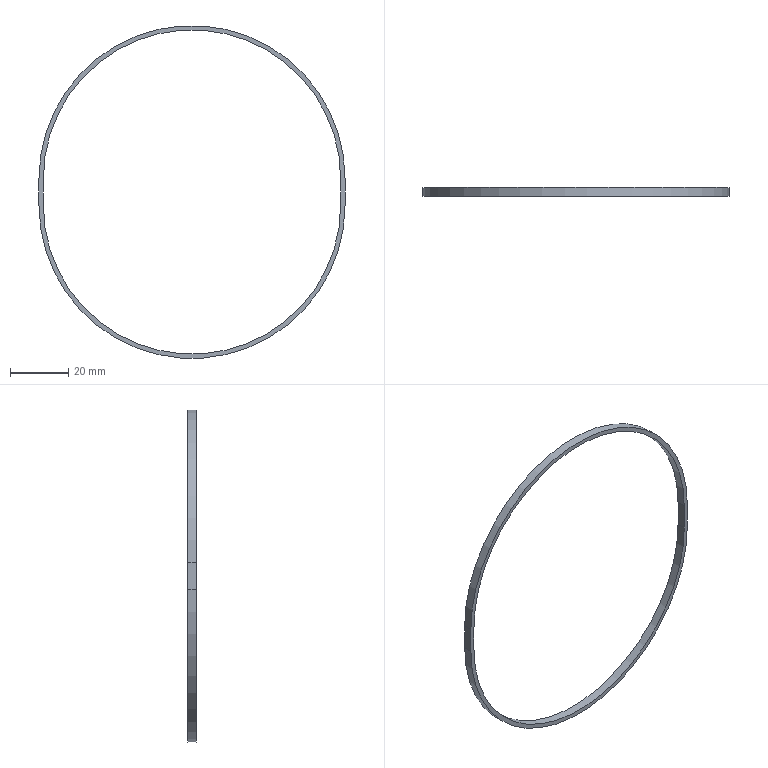Part | STEP file | 1-56.26 | 1 solid | 10 faces | box 105 x 3 x 114.181 mm | volume 1546 mm3 | plane 6 | cylinder 4 | commonest cylinder face diameters 102 x2 105 x2
STEP:
#1=CARTESIAN_POINT('',(0.,0.,0.));
#2=DIRECTION('',(0.,0.,1.));
#3=DIRECTION('',(1.,0.,0.));
#4=AXIS2_PLACEMENT_3D('',#1,#2,#3);
#5=CARTESIAN_POINT('',(-52.5,0.,-9.181));
#6=VERTEX_POINT('',#5);
#7=CARTESIAN_POINT('',(52.5,0.,-9.181));
#8=VERTEX_POINT('',#7);
#9=CARTESIAN_POINT('',(0.,0.,-9.181));
#10=DIRECTION('',(0.,-1.,0.));
#11=DIRECTION('',(-1.,0.,0.));
#12=AXIS2_PLACEMENT_3D('',#9,#10,#11);
#13=CIRCLE('',#12,52.5);
#14=CARTESIAN_POINT('',(4.591,0.,-4.591));
#15=DIRECTION('',(0.,-1.,0.));
#16=DIRECTION('',(1.,0.,0.));
#17=AXIS2_PLACEMENT_3D('',#14,#15,#16);
#18=PLANE('',#17);
#19=CARTESIAN_POINT('',(-4.591,-4.591));
#20=DIRECTION('',(-1.,0.));
#21=AXIS2_PLACEMENT_2D('',#19,#20);
#22=CIRCLE('',#21,52.5);
#23=(GEOMETRIC_REPRESENTATION_CONTEXT(2)PARAMETRIC_REPRESENTATION_CONTEXT()REPRESENTATION_CONTEXT('',''));
#24=DEFINITIONAL_REPRESENTATION('',(#22),#23);
#25=PCURVE('',#18,#24);
#26=CARTESIAN_POINT('',(0.,0.,-9.181));
#27=DIRECTION('',(0.,1.,0.));
#28=DIRECTION('',(-1.,0.,0.));
#29=AXIS2_PLACEMENT_3D('',#26,#27,#28);
#30=CYLINDRICAL_SURFACE('',#29,52.5);
#31=CARTESIAN_POINT('',(6.283,0.));
#32=DIRECTION('',(-1.,0.));
#33=VECTOR('',#32,1.);
#34=LINE('',#31,#33);
#35=(GEOMETRIC_REPRESENTATION_CONTEXT(2)PARAMETRIC_REPRESENTATION_CONTEXT()REPRESENTATION_CONTEXT('',''));
#36=DEFINITIONAL_REPRESENTATION('',(#34),#35);
#37=PCURVE('',#30,#36);
#38=SURFACE_CURVE('',#13,(#25,#37),.PCURVE_S1.);
#39=EDGE_CURVE('',#6,#8,#38,.T.);
#40=ORIENTED_EDGE('',*,*,#39,.T.);
#41=CARTESIAN_POINT('',(52.5,0.,0.));
#42=VERTEX_POINT('',#41);
#43=CARTESIAN_POINT('',(52.5,0.,-9.181));
#44=DIRECTION('',(0.,0.,1.));
#45=VECTOR('',#44,1.);
#46=LINE('',#43,#45);
#47=CARTESIAN_POINT('',(47.909,-4.591));
#48=DIRECTION('',(0.,1.));
#49=VECTOR('',#48,1.);
#50=LINE('',#47,#49);
#51=(GEOMETRIC_REPRESENTATION_CONTEXT(2)PARAMETRIC_REPRESENTATION_CONTEXT()REPRESENTATION_CONTEXT('',''));
#52=DEFINITIONAL_REPRESENTATION('',(#50),#51);
#53=PCURVE('',#18,#52);
#54=CARTESIAN_POINT('',(52.5,1.5,-4.591));
#55=DIRECTION('',(-1.,0.,0.));
#56=DIRECTION('',(0.,0.,1.));
#57=AXIS2_PLACEMENT_3D('',#54,#55,#56);
#58=PLANE('',#57);
#59=CARTESIAN_POINT('',(-4.591,-1.5));
#60=DIRECTION('',(1.,0.));
#61=VECTOR('',#60,1.);
#62=LINE('',#59,#61);
#63=(GEOMETRIC_REPRESENTATION_CONTEXT(2)PARAMETRIC_REPRESENTATION_CONTEXT()REPRESENTATION_CONTEXT('',''));
#64=DEFINITIONAL_REPRESENTATION('',(#62),#63);
#65=PCURVE('',#58,#64);
#66=SURFACE_CURVE('',#46,(#53,#65),.PCURVE_S1.);
#67=EDGE_CURVE('',#8,#42,#66,.T.);
#68=ORIENTED_EDGE('',*,*,#67,.T.);
#69=CARTESIAN_POINT('',(-52.5,0.,0.));
#70=VERTEX_POINT('',#69);
#71=CARTESIAN_POINT('',(0.,0.,0.));
#72=DIRECTION('',(0.,-1.,0.));
#73=DIRECTION('',(1.,0.,0.));
#74=AXIS2_PLACEMENT_3D('',#71,#72,#73);
#75=CIRCLE('',#74,52.5);
#76=CARTESIAN_POINT('',(-4.591,4.591));
#77=DIRECTION('',(1.,0.));
#78=AXIS2_PLACEMENT_2D('',#76,#77);
#79=CIRCLE('',#78,52.5);
#80=(GEOMETRIC_REPRESENTATION_CONTEXT(2)PARAMETRIC_REPRESENTATION_CONTEXT()REPRESENTATION_CONTEXT('',''));
#81=DEFINITIONAL_REPRESENTATION('',(#79),#80);
#82=PCURVE('',#18,#81);
#83=CARTESIAN_POINT('',(0.,0.,0.));
#84=DIRECTION('',(0.,1.,0.));
#85=DIRECTION('',(1.,0.,0.));
#86=AXIS2_PLACEMENT_3D('',#83,#84,#85);
#87=CYLINDRICAL_SURFACE('',#86,52.5);
#88=CARTESIAN_POINT('',(6.283,0.));
#89=DIRECTION('',(-1.,0.));
#90=VECTOR('',#89,1.);
#91=LINE('',#88,#90);
#92=(GEOMETRIC_REPRESENTATION_CONTEXT(2)PARAMETRIC_REPRESENTATION_CONTEXT()REPRESENTATION_CONTEXT('',''));
#93=DEFINITIONAL_REPRESENTATION('',(#91),#92);
#94=PCURVE('',#87,#93);
#95=SURFACE_CURVE('',#75,(#82,#94),.PCURVE_S1.);
#96=EDGE_CURVE('',#42,#70,#95,.T.);
#97=ORIENTED_EDGE('',*,*,#96,.T.);
#98=CARTESIAN_POINT('',(-52.5,0.,0.));
#99=DIRECTION('',(0.,0.,-1.));
#100=VECTOR('',#99,1.);
#101=LINE('',#98,#100);
#102=CARTESIAN_POINT('',(-57.091,4.591));
#103=DIRECTION('',(0.,-1.));
#104=VECTOR('',#103,1.);
#105=LINE('',#102,#104);
#106=(GEOMETRIC_REPRESENTATION_CONTEXT(2)PARAMETRIC_REPRESENTATION_CONTEXT()REPRESENTATION_CONTEXT('',''));
#107=DEFINITIONAL_REPRESENTATION('',(#105),#106);
#108=PCURVE('',#18,#107);
#109=CARTESIAN_POINT('',(-52.5,1.5,-4.591));
#110=DIRECTION('',(1.,0.,0.));
#111=DIRECTION('',(0.,0.,-1.));
#112=AXIS2_PLACEMENT_3D('',#109,#110,#111);
#113=PLANE('',#112);
#114=CARTESIAN_POINT('',(-4.591,-1.5));
#115=DIRECTION('',(1.,0.));
#116=VECTOR('',#115,1.);
#117=LINE('',#114,#116);
#118=(GEOMETRIC_REPRESENTATION_CONTEXT(2)PARAMETRIC_REPRESENTATION_CONTEXT()REPRESENTATION_CONTEXT('',''));
#119=DEFINITIONAL_REPRESENTATION('',(#117),#118);
#120=PCURVE('',#113,#119);
#121=SURFACE_CURVE('',#101,(#108,#120),.PCURVE_S1.);
#122=EDGE_CURVE('',#70,#6,#121,.T.);
#123=ORIENTED_EDGE('',*,*,#122,.T.);
#124=EDGE_LOOP('',(#40,#68,#97,#123));
#125=FACE_BOUND('',#124,.T.);
#126=CARTESIAN_POINT('',(51.,0.,0.));
#127=VERTEX_POINT('',#126);
#128=CARTESIAN_POINT('',(51.,0.,-9.181));
#129=VERTEX_POINT('',#128);
#130=CARTESIAN_POINT('',(51.,0.,0.));
#131=DIRECTION('',(0.,0.,-1.));
#132=VECTOR('',#131,1.);
#133=LINE('',#130,#132);
#134=CARTESIAN_POINT('',(46.409,4.591));
#135=DIRECTION('',(0.,-1.));
#136=VECTOR('',#135,1.);
#137=LINE('',#134,#136);
#138=(GEOMETRIC_REPRESENTATION_CONTEXT(2)PARAMETRIC_REPRESENTATION_CONTEXT()REPRESENTATION_CONTEXT('',''));
#139=DEFINITIONAL_REPRESENTATION('',(#137),#138);
#140=PCURVE('',#18,#139);
#141=CARTESIAN_POINT('',(51.,1.5,-4.591));
#142=DIRECTION('',(1.,0.,0.));
#143=DIRECTION('',(0.,0.,-1.));
#144=AXIS2_PLACEMENT_3D('',#141,#142,#143);
#145=PLANE('',#144);
#146=CARTESIAN_POINT('',(-4.591,-1.5));
#147=DIRECTION('',(1.,0.));
#148=VECTOR('',#147,1.);
#149=LINE('',#146,#148);
#150=(GEOMETRIC_REPRESENTATION_CONTEXT(2)PARAMETRIC_REPRESENTATION_CONTEXT()REPRESENTATION_CONTEXT('',''));
#151=DEFINITIONAL_REPRESENTATION('',(#149),#150);
#152=PCURVE('',#145,#151);
#153=SURFACE_CURVE('',#133,(#140,#152),.PCURVE_S1.);
#154=EDGE_CURVE('',#127,#129,#153,.T.);
#155=ORIENTED_EDGE('',*,*,#154,.T.);
#156=CARTESIAN_POINT('',(-51.,0.,-9.181));
#157=VERTEX_POINT('',#156);
#158=CARTESIAN_POINT('',(0.,0.,-9.181));
#159=DIRECTION('',(0.,1.,0.));
#160=DIRECTION('',(1.,0.,0.));
#161=AXIS2_PLACEMENT_3D('',#158,#159,#160);
#162=CIRCLE('',#161,51.);
#163=CARTESIAN_POINT('',(46.409,-4.591));
#164=CARTESIAN_POINT('',(46.409,-92.925));
#165=CARTESIAN_POINT('',(-30.091,-48.758));
#166=CARTESIAN_POINT('',(-106.591,-4.591));
#167=CARTESIAN_POINT('',(-30.091,39.577));
#168=CARTESIAN_POINT('',(46.409,83.744));
#169=CARTESIAN_POINT('',(46.409,-4.591));
#170=(BOUNDED_CURVE()B_SPLINE_CURVE(2,(#163,#164,#165,#166,#167,#168,#169),.UNSPECIFIED.,.T.,.F.)B_SPLINE_CURVE_WITH_KNOTS((1,2,2,2,2,1),(-2.094,0.,2.094,4.189,6.283,8.378),.UNSPECIFIED.)CURVE()GEOMETRIC_REPRESENTATION_ITEM()RATIONAL_B_SPLINE_CURVE((1.,0.5,1.,0.5,1.,0.5,1.))REPRESENTATION_ITEM(''));
#171=(GEOMETRIC_REPRESENTATION_CONTEXT(2)PARAMETRIC_REPRESENTATION_CONTEXT()REPRESENTATION_CONTEXT('',''));
#172=DEFINITIONAL_REPRESENTATION('',(#170),#171);
#173=PCURVE('',#18,#172);
#174=CARTESIAN_POINT('',(0.,0.,-9.181));
#175=DIRECTION('',(0.,1.,0.));
#176=DIRECTION('',(1.,0.,0.));
#177=AXIS2_PLACEMENT_3D('',#174,#175,#176);
#178=CYLINDRICAL_SURFACE('',#177,51.);
#179=CARTESIAN_POINT('',(0.,0.));
#180=DIRECTION('',(1.,0.));
#181=VECTOR('',#180,1.);
#182=LINE('',#179,#181);
#183=(GEOMETRIC_REPRESENTATION_CONTEXT(2)PARAMETRIC_REPRESENTATION_CONTEXT()REPRESENTATION_CONTEXT('',''));
#184=DEFINITIONAL_REPRESENTATION('',(#182),#183);
#185=PCURVE('',#178,#184);
#186=SURFACE_CURVE('',#162,(#173,#185),.PCURVE_S1.);
#187=EDGE_CURVE('',#129,#157,#186,.T.);
#188=ORIENTED_EDGE('',*,*,#187,.T.);
#189=CARTESIAN_POINT('',(-51.,0.,0.));
#190=VERTEX_POINT('',#189);
#191=CARTESIAN_POINT('',(-51.,0.,-9.181));
#192=DIRECTION('',(0.,0.,1.));
#193=VECTOR('',#192,1.);
#194=LINE('',#191,#193);
#195=CARTESIAN_POINT('',(-55.591,-4.591));
#196=DIRECTION('',(0.,1.));
#197=VECTOR('',#196,1.);
#198=LINE('',#195,#197);
#199=(GEOMETRIC_REPRESENTATION_CONTEXT(2)PARAMETRIC_REPRESENTATION_CONTEXT()REPRESENTATION_CONTEXT('',''));
#200=DEFINITIONAL_REPRESENTATION('',(#198),#199);
#201=PCURVE('',#18,#200);
#202=CARTESIAN_POINT('',(-51.,1.5,-4.591));
#203=DIRECTION('',(-1.,0.,0.));
#204=DIRECTION('',(0.,0.,1.));
#205=AXIS2_PLACEMENT_3D('',#202,#203,#204);
#206=PLANE('',#205);
#207=CARTESIAN_POINT('',(-4.591,-1.5));
#208=DIRECTION('',(1.,0.));
#209=VECTOR('',#208,1.);
#210=LINE('',#207,#209);
#211=(GEOMETRIC_REPRESENTATION_CONTEXT(2)PARAMETRIC_REPRESENTATION_CONTEXT()REPRESENTATION_CONTEXT('',''));
#212=DEFINITIONAL_REPRESENTATION('',(#210),#211);
#213=PCURVE('',#206,#212);
#214=SURFACE_CURVE('',#194,(#201,#213),.PCURVE_S1.);
#215=EDGE_CURVE('',#157,#190,#214,.T.);
#216=ORIENTED_EDGE('',*,*,#215,.T.);
#217=CARTESIAN_POINT('',(0.,0.,0.));
#218=DIRECTION('',(0.,1.,0.));
#219=DIRECTION('',(-1.,0.,0.));
#220=AXIS2_PLACEMENT_3D('',#217,#218,#219);
#221=CIRCLE('',#220,51.);
#222=CARTESIAN_POINT('',(-55.591,4.591));
#223=CARTESIAN_POINT('',(-55.591,92.925));
#224=CARTESIAN_POINT('',(20.909,48.758));
#225=CARTESIAN_POINT('',(97.409,4.591));
#226=CARTESIAN_POINT('',(20.909,-39.577));
#227=CARTESIAN_POINT('',(-55.591,-83.744));
#228=CARTESIAN_POINT('',(-55.591,4.591));
#229=(BOUNDED_CURVE()B_SPLINE_CURVE(2,(#222,#223,#224,#225,#226,#227,#228),.UNSPECIFIED.,.T.,.F.)B_SPLINE_CURVE_WITH_KNOTS((1,2,2,2,2,1),(-2.094,0.,2.094,4.189,6.283,8.378),.UNSPECIFIED.)CURVE()GEOMETRIC_REPRESENTATION_ITEM()RATIONAL_B_SPLINE_CURVE((1.,0.5,1.,0.5,1.,0.5,1.))REPRESENTATION_ITEM(''));
#230=(GEOMETRIC_REPRESENTATION_CONTEXT(2)PARAMETRIC_REPRESENTATION_CONTEXT()REPRESENTATION_CONTEXT('',''));
#231=DEFINITIONAL_REPRESENTATION('',(#229),#230);
#232=PCURVE('',#18,#231);
#233=CARTESIAN_POINT('',(0.,0.,0.));
#234=DIRECTION('',(0.,1.,0.));
#235=DIRECTION('',(-1.,0.,0.));
#236=AXIS2_PLACEMENT_3D('',#233,#234,#235);
#237=CYLINDRICAL_SURFACE('',#236,51.);
#238=CARTESIAN_POINT('',(0.,0.));
#239=DIRECTION('',(1.,0.));
#240=VECTOR('',#239,1.);
#241=LINE('',#238,#240);
#242=(GEOMETRIC_REPRESENTATION_CONTEXT(2)PARAMETRIC_REPRESENTATION_CONTEXT()REPRESENTATION_CONTEXT('',''));
#243=DEFINITIONAL_REPRESENTATION('',(#241),#242);
#244=PCURVE('',#237,#243);
#245=SURFACE_CURVE('',#221,(#232,#244),.PCURVE_S1.);
#246=EDGE_CURVE('',#190,#127,#245,.T.);
#247=ORIENTED_EDGE('',*,*,#246,.T.);
#248=EDGE_LOOP('',(#155,#188,#216,#247));
#249=FACE_BOUND('',#248,.T.);
#250=ADVANCED_FACE('',(#125,#249),#18,.T.);
#251=CARTESIAN_POINT('',(-52.5,3.,-9.181));
#252=VERTEX_POINT('',#251);
#253=CARTESIAN_POINT('',(52.5,3.,-9.181));
#254=VERTEX_POINT('',#253);
#255=CARTESIAN_POINT('',(0.,3.,-9.181));
#256=DIRECTION('',(0.,-1.,0.));
#257=DIRECTION('',(-1.,0.,0.));
#258=AXIS2_PLACEMENT_3D('',#255,#256,#257);
#259=CIRCLE('',#258,52.5);
#260=CARTESIAN_POINT('',(4.591,3.,-4.591));
#261=DIRECTION('',(0.,-1.,0.));
#262=DIRECTION('',(1.,0.,0.));
#263=AXIS2_PLACEMENT_3D('',#260,#261,#262);
#264=PLANE('',#263);
#265=CARTESIAN_POINT('',(-4.591,-4.591));
#266=DIRECTION('',(-1.,0.));
#267=AXIS2_PLACEMENT_2D('',#265,#266);
#268=CIRCLE('',#267,52.5);
#269=(GEOMETRIC_REPRESENTATION_CONTEXT(2)PARAMETRIC_REPRESENTATION_CONTEXT()REPRESENTATION_CONTEXT('',''));
#270=DEFINITIONAL_REPRESENTATION('',(#268),#269);
#271=PCURVE('',#264,#270);
#272=CARTESIAN_POINT('',(6.283,3.));
#273=DIRECTION('',(-1.,0.));
#274=VECTOR('',#273,1.);
#275=LINE('',#272,#274);
#276=(GEOMETRIC_REPRESENTATION_CONTEXT(2)PARAMETRIC_REPRESENTATION_CONTEXT()REPRESENTATION_CONTEXT('',''));
#277=DEFINITIONAL_REPRESENTATION('',(#275),#276);
#278=PCURVE('',#30,#277);
#279=SURFACE_CURVE('',#259,(#271,#278),.PCURVE_S1.);
#280=EDGE_CURVE('',#252,#254,#279,.T.);
#281=ORIENTED_EDGE('',*,*,#280,.T.);
#282=CARTESIAN_POINT('',(52.5,3.,0.));
#283=VERTEX_POINT('',#282);
#284=CARTESIAN_POINT('',(52.5,3.,-9.181));
#285=DIRECTION('',(0.,0.,1.));
#286=VECTOR('',#285,1.);
#287=LINE('',#284,#286);
#288=CARTESIAN_POINT('',(47.909,-4.591));
#289=DIRECTION('',(0.,1.));
#290=VECTOR('',#289,1.);
#291=LINE('',#288,#290);
#292=(GEOMETRIC_REPRESENTATION_CONTEXT(2)PARAMETRIC_REPRESENTATION_CONTEXT()REPRESENTATION_CONTEXT('',''));
#293=DEFINITIONAL_REPRESENTATION('',(#291),#292);
#294=PCURVE('',#264,#293);
#295=CARTESIAN_POINT('',(-4.591,1.5));
#296=DIRECTION('',(1.,0.));
#297=VECTOR('',#296,1.);
#298=LINE('',#295,#297);
#299=(GEOMETRIC_REPRESENTATION_CONTEXT(2)PARAMETRIC_REPRESENTATION_CONTEXT()REPRESENTATION_CONTEXT('',''));
#300=DEFINITIONAL_REPRESENTATION('',(#298),#299);
#301=PCURVE('',#58,#300);
#302=SURFACE_CURVE('',#287,(#294,#301),.PCURVE_S1.);
#303=EDGE_CURVE('',#254,#283,#302,.T.);
#304=ORIENTED_EDGE('',*,*,#303,.T.);
#305=CARTESIAN_POINT('',(-52.5,3.,0.));
#306=VERTEX_POINT('',#305);
#307=CARTESIAN_POINT('',(0.,3.,0.));
#308=DIRECTION('',(0.,-1.,0.));
#309=DIRECTION('',(1.,0.,0.));
#310=AXIS2_PLACEMENT_3D('',#307,#308,#309);
#311=CIRCLE('',#310,52.5);
#312=CARTESIAN_POINT('',(-4.591,4.591));
#313=DIRECTION('',(1.,0.));
#314=AXIS2_PLACEMENT_2D('',#312,#313);
#315=CIRCLE('',#314,52.5);
#316=(GEOMETRIC_REPRESENTATION_CONTEXT(2)PARAMETRIC_REPRESENTATION_CONTEXT()REPRESENTATION_CONTEXT('',''));
#317=DEFINITIONAL_REPRESENTATION('',(#315),#316);
#318=PCURVE('',#264,#317);
#319=CARTESIAN_POINT('',(6.283,3.));
#320=DIRECTION('',(-1.,0.));
#321=VECTOR('',#320,1.);
#322=LINE('',#319,#321);
#323=(GEOMETRIC_REPRESENTATION_CONTEXT(2)PARAMETRIC_REPRESENTATION_CONTEXT()REPRESENTATION_CONTEXT('',''));
#324=DEFINITIONAL_REPRESENTATION('',(#322),#323);
#325=PCURVE('',#87,#324);
#326=SURFACE_CURVE('',#311,(#318,#325),.PCURVE_S1.);
#327=EDGE_CURVE('',#283,#306,#326,.T.);
#328=ORIENTED_EDGE('',*,*,#327,.T.);
#329=CARTESIAN_POINT('',(-52.5,3.,0.));
#330=DIRECTION('',(0.,0.,-1.));
#331=VECTOR('',#330,1.);
#332=LINE('',#329,#331);
#333=CARTESIAN_POINT('',(-57.091,4.591));
#334=DIRECTION('',(0.,-1.));
#335=VECTOR('',#334,1.);
#336=LINE('',#333,#335);
#337=(GEOMETRIC_REPRESENTATION_CONTEXT(2)PARAMETRIC_REPRESENTATION_CONTEXT()REPRESENTATION_CONTEXT('',''));
#338=DEFINITIONAL_REPRESENTATION('',(#336),#337);
#339=PCURVE('',#264,#338);
#340=CARTESIAN_POINT('',(-4.591,1.5));
#341=DIRECTION('',(1.,0.));
#342=VECTOR('',#341,1.);
#343=LINE('',#340,#342);
#344=(GEOMETRIC_REPRESENTATION_CONTEXT(2)PARAMETRIC_REPRESENTATION_CONTEXT()REPRESENTATION_CONTEXT('',''));
#345=DEFINITIONAL_REPRESENTATION('',(#343),#344);
#346=PCURVE('',#113,#345);
#347=SURFACE_CURVE('',#332,(#339,#346),.PCURVE_S1.);
#348=EDGE_CURVE('',#306,#252,#347,.T.);
#349=ORIENTED_EDGE('',*,*,#348,.T.);
#350=EDGE_LOOP('',(#281,#304,#328,#349));
#351=FACE_BOUND('',#350,.F.);
#352=CARTESIAN_POINT('',(51.,3.,0.));
#353=VERTEX_POINT('',#352);
#354=CARTESIAN_POINT('',(51.,3.,-9.181));
#355=VERTEX_POINT('',#354);
#356=CARTESIAN_POINT('',(51.,3.,0.));
#357=DIRECTION('',(0.,0.,-1.));
#358=VECTOR('',#357,1.);
#359=LINE('',#356,#358);
#360=CARTESIAN_POINT('',(46.409,4.591));
#361=DIRECTION('',(0.,-1.));
#362=VECTOR('',#361,1.);
#363=LINE('',#360,#362);
#364=(GEOMETRIC_REPRESENTATION_CONTEXT(2)PARAMETRIC_REPRESENTATION_CONTEXT()REPRESENTATION_CONTEXT('',''));
#365=DEFINITIONAL_REPRESENTATION('',(#363),#364);
#366=PCURVE('',#264,#365);
#367=CARTESIAN_POINT('',(-4.591,1.5));
#368=DIRECTION('',(1.,0.));
#369=VECTOR('',#368,1.);
#370=LINE('',#367,#369);
#371=(GEOMETRIC_REPRESENTATION_CONTEXT(2)PARAMETRIC_REPRESENTATION_CONTEXT()REPRESENTATION_CONTEXT('',''));
#372=DEFINITIONAL_REPRESENTATION('',(#370),#371);
#373=PCURVE('',#145,#372);
#374=SURFACE_CURVE('',#359,(#366,#373),.PCURVE_S1.);
#375=EDGE_CURVE('',#353,#355,#374,.T.);
#376=ORIENTED_EDGE('',*,*,#375,.T.);
#377=CARTESIAN_POINT('',(-51.,3.,-9.181));
#378=VERTEX_POINT('',#377);
#379=CARTESIAN_POINT('',(0.,3.,-9.181));
#380=DIRECTION('',(0.,1.,0.));
#381=DIRECTION('',(1.,0.,0.));
#382=AXIS2_PLACEMENT_3D('',#379,#380,#381);
#383=CIRCLE('',#382,51.);
#384=CARTESIAN_POINT('',(46.409,-4.591));
#385=CARTESIAN_POINT('',(46.409,-92.925));
#386=CARTESIAN_POINT('',(-30.091,-48.758));
#387=CARTESIAN_POINT('',(-106.591,-4.591));
#388=CARTESIAN_POINT('',(-30.091,39.577));
#389=CARTESIAN_POINT('',(46.409,83.744));
#390=CARTESIAN_POINT('',(46.409,-4.591));
#391=(BOUNDED_CURVE()B_SPLINE_CURVE(2,(#384,#385,#386,#387,#388,#389,#390),.UNSPECIFIED.,.T.,.F.)B_SPLINE_CURVE_WITH_KNOTS((1,2,2,2,2,1),(-2.094,0.,2.094,4.189,6.283,8.378),.UNSPECIFIED.)CURVE()GEOMETRIC_REPRESENTATION_ITEM()RATIONAL_B_SPLINE_CURVE((1.,0.5,1.,0.5,1.,0.5,1.))REPRESENTATION_ITEM(''));
#392=(GEOMETRIC_REPRESENTATION_CONTEXT(2)PARAMETRIC_REPRESENTATION_CONTEXT()REPRESENTATION_CONTEXT('',''));
#393=DEFINITIONAL_REPRESENTATION('',(#391),#392);
#394=PCURVE('',#264,#393);
#395=CARTESIAN_POINT('',(0.,3.));
#396=DIRECTION('',(1.,0.));
#397=VECTOR('',#396,1.);
#398=LINE('',#395,#397);
#399=(GEOMETRIC_REPRESENTATION_CONTEXT(2)PARAMETRIC_REPRESENTATION_CONTEXT()REPRESENTATION_CONTEXT('',''));
#400=DEFINITIONAL_REPRESENTATION('',(#398),#399);
#401=PCURVE('',#178,#400);
#402=SURFACE_CURVE('',#383,(#394,#401),.PCURVE_S1.);
#403=EDGE_CURVE('',#355,#378,#402,.T.);
#404=ORIENTED_EDGE('',*,*,#403,.T.);
#405=CARTESIAN_POINT('',(-51.,3.,0.));
#406=VERTEX_POINT('',#405);
#407=CARTESIAN_POINT('',(-51.,3.,-9.181));
#408=DIRECTION('',(0.,0.,1.));
#409=VECTOR('',#408,1.);
#410=LINE('',#407,#409);
#411=CARTESIAN_POINT('',(-55.591,-4.591));
#412=DIRECTION('',(0.,1.));
#413=VECTOR('',#412,1.);
#414=LINE('',#411,#413);
#415=(GEOMETRIC_REPRESENTATION_CONTEXT(2)PARAMETRIC_REPRESENTATION_CONTEXT()REPRESENTATION_CONTEXT('',''));
#416=DEFINITIONAL_REPRESENTATION('',(#414),#415);
#417=PCURVE('',#264,#416);
#418=CARTESIAN_POINT('',(-4.591,1.5));
#419=DIRECTION('',(1.,0.));
#420=VECTOR('',#419,1.);
#421=LINE('',#418,#420);
#422=(GEOMETRIC_REPRESENTATION_CONTEXT(2)PARAMETRIC_REPRESENTATION_CONTEXT()REPRESENTATION_CONTEXT('',''));
#423=DEFINITIONAL_REPRESENTATION('',(#421),#422);
#424=PCURVE('',#206,#423);
#425=SURFACE_CURVE('',#410,(#417,#424),.PCURVE_S1.);
#426=EDGE_CURVE('',#378,#406,#425,.T.);
#427=ORIENTED_EDGE('',*,*,#426,.T.);
#428=CARTESIAN_POINT('',(0.,3.,0.));
#429=DIRECTION('',(0.,1.,0.));
#430=DIRECTION('',(-1.,0.,0.));
#431=AXIS2_PLACEMENT_3D('',#428,#429,#430);
#432=CIRCLE('',#431,51.);
#433=CARTESIAN_POINT('',(-55.591,4.591));
#434=CARTESIAN_POINT('',(-55.591,92.925));
#435=CARTESIAN_POINT('',(20.909,48.758));
#436=CARTESIAN_POINT('',(97.409,4.591));
#437=CARTESIAN_POINT('',(20.909,-39.577));
#438=CARTESIAN_POINT('',(-55.591,-83.744));
#439=CARTESIAN_POINT('',(-55.591,4.591));
#440=(BOUNDED_CURVE()B_SPLINE_CURVE(2,(#433,#434,#435,#436,#437,#438,#439),.UNSPECIFIED.,.T.,.F.)B_SPLINE_CURVE_WITH_KNOTS((1,2,2,2,2,1),(-2.094,0.,2.094,4.189,6.283,8.378),.UNSPECIFIED.)CURVE()GEOMETRIC_REPRESENTATION_ITEM()RATIONAL_B_SPLINE_CURVE((1.,0.5,1.,0.5,1.,0.5,1.))REPRESENTATION_ITEM(''));
#441=(GEOMETRIC_REPRESENTATION_CONTEXT(2)PARAMETRIC_REPRESENTATION_CONTEXT()REPRESENTATION_CONTEXT('',''));
#442=DEFINITIONAL_REPRESENTATION('',(#440),#441);
#443=PCURVE('',#264,#442);
#444=CARTESIAN_POINT('',(0.,3.));
#445=DIRECTION('',(1.,0.));
#446=VECTOR('',#445,1.);
#447=LINE('',#444,#446);
#448=(GEOMETRIC_REPRESENTATION_CONTEXT(2)PARAMETRIC_REPRESENTATION_CONTEXT()REPRESENTATION_CONTEXT('',''));
#449=DEFINITIONAL_REPRESENTATION('',(#447),#448);
#450=PCURVE('',#237,#449);
#451=SURFACE_CURVE('',#432,(#443,#450),.PCURVE_S1.);
#452=EDGE_CURVE('',#406,#353,#451,.T.);
#453=ORIENTED_EDGE('',*,*,#452,.T.);
#454=EDGE_LOOP('',(#376,#404,#427,#453));
#455=FACE_BOUND('',#454,.F.);
#456=ADVANCED_FACE('',(#351,#455),#264,.F.);
#457=CARTESIAN_POINT('',(-52.5,0.,-9.181));
#458=DIRECTION('',(0.,1.,0.));
#459=VECTOR('',#458,1.);
#460=LINE('',#457,#459);
#461=CARTESIAN_POINT('',(6.283,0.));
#462=DIRECTION('',(0.,1.));
#463=VECTOR('',#462,1.);
#464=LINE('',#461,#463);
#465=(GEOMETRIC_REPRESENTATION_CONTEXT(2)PARAMETRIC_REPRESENTATION_CONTEXT()REPRESENTATION_CONTEXT('',''));
#466=DEFINITIONAL_REPRESENTATION('',(#464),#465);
#467=PCURVE('',#30,#466);
#468=CARTESIAN_POINT('',(4.591,-1.5));
#469=DIRECTION('',(0.,1.));
#470=VECTOR('',#469,1.);
#471=LINE('',#468,#470);
#472=(GEOMETRIC_REPRESENTATION_CONTEXT(2)PARAMETRIC_REPRESENTATION_CONTEXT()REPRESENTATION_CONTEXT('',''));
#473=DEFINITIONAL_REPRESENTATION('',(#471),#472);
#474=PCURVE('',#113,#473);
#475=SURFACE_CURVE('',#460,(#467,#474),.PCURVE_S1.);
#476=EDGE_CURVE('',#6,#252,#475,.T.);
#477=ORIENTED_EDGE('',*,*,#476,.T.);
#478=ORIENTED_EDGE('',*,*,#280,.T.);
#479=CARTESIAN_POINT('',(52.5,0.,-9.181));
#480=DIRECTION('',(0.,1.,0.));
#481=VECTOR('',#480,1.);
#482=LINE('',#479,#481);
#483=CARTESIAN_POINT('',(3.142,0.));
#484=DIRECTION('',(0.,1.));
#485=VECTOR('',#484,1.);
#486=LINE('',#483,#485);
#487=(GEOMETRIC_REPRESENTATION_CONTEXT(2)PARAMETRIC_REPRESENTATION_CONTEXT()REPRESENTATION_CONTEXT('',''));
#488=DEFINITIONAL_REPRESENTATION('',(#486),#487);
#489=PCURVE('',#30,#488);
#490=CARTESIAN_POINT('',(-4.591,-1.5));
#491=DIRECTION('',(0.,1.));
#492=VECTOR('',#491,1.);
#493=LINE('',#490,#492);
#494=(GEOMETRIC_REPRESENTATION_CONTEXT(2)PARAMETRIC_REPRESENTATION_CONTEXT()REPRESENTATION_CONTEXT('',''));
#495=DEFINITIONAL_REPRESENTATION('',(#493),#494);
#496=PCURVE('',#58,#495);
#497=SURFACE_CURVE('',#482,(#489,#496),.PCURVE_S1.);
#498=EDGE_CURVE('',#8,#254,#497,.T.);
#499=ORIENTED_EDGE('',*,*,#498,.F.);
#500=ORIENTED_EDGE('',*,*,#39,.F.);
#501=EDGE_LOOP('',(#477,#478,#499,#500));
#502=FACE_BOUND('',#501,.T.);
#503=ADVANCED_FACE('',(#502),#30,.T.);
#504=ORIENTED_EDGE('',*,*,#67,.T.);
#505=CARTESIAN_POINT('',(52.5,0.,0.));
#506=DIRECTION('',(0.,1.,0.));
#507=VECTOR('',#506,1.);
#508=LINE('',#505,#507);
#509=CARTESIAN_POINT('',(4.591,-1.5));
#510=DIRECTION('',(0.,1.));
#511=VECTOR('',#510,1.);
#512=LINE('',#509,#511);
#513=(GEOMETRIC_REPRESENTATION_CONTEXT(2)PARAMETRIC_REPRESENTATION_CONTEXT()REPRESENTATION_CONTEXT('',''));
#514=DEFINITIONAL_REPRESENTATION('',(#512),#513);
#515=PCURVE('',#58,#514);
#516=CARTESIAN_POINT('',(6.283,0.));
#517=DIRECTION('',(0.,1.));
#518=VECTOR('',#517,1.);
#519=LINE('',#516,#518);
#520=(GEOMETRIC_REPRESENTATION_CONTEXT(2)PARAMETRIC_REPRESENTATION_CONTEXT()REPRESENTATION_CONTEXT('',''));
#521=DEFINITIONAL_REPRESENTATION('',(#519),#520);
#522=PCURVE('',#87,#521);
#523=SURFACE_CURVE('',#508,(#515,#522),.PCURVE_S1.);
#524=EDGE_CURVE('',#42,#283,#523,.T.);
#525=ORIENTED_EDGE('',*,*,#524,.T.);
#526=ORIENTED_EDGE('',*,*,#303,.F.);
#527=ORIENTED_EDGE('',*,*,#498,.F.);
#528=EDGE_LOOP('',(#504,#525,#526,#527));
#529=FACE_BOUND('',#528,.F.);
#530=ADVANCED_FACE('',(#529),#58,.F.);
#531=ORIENTED_EDGE('',*,*,#524,.T.);
#532=ORIENTED_EDGE('',*,*,#327,.T.);
#533=CARTESIAN_POINT('',(-52.5,0.,0.));
#534=DIRECTION('',(0.,1.,0.));
#535=VECTOR('',#534,1.);
#536=LINE('',#533,#535);
#537=CARTESIAN_POINT('',(3.142,0.));
#538=DIRECTION('',(0.,1.));
#539=VECTOR('',#538,1.);
#540=LINE('',#537,#539);
#541=(GEOMETRIC_REPRESENTATION_CONTEXT(2)PARAMETRIC_REPRESENTATION_CONTEXT()REPRESENTATION_CONTEXT('',''));
#542=DEFINITIONAL_REPRESENTATION('',(#540),#541);
#543=PCURVE('',#87,#542);
#544=CARTESIAN_POINT('',(-4.591,-1.5));
#545=DIRECTION('',(0.,1.));
#546=VECTOR('',#545,1.);
#547=LINE('',#544,#546);
#548=(GEOMETRIC_REPRESENTATION_CONTEXT(2)PARAMETRIC_REPRESENTATION_CONTEXT()REPRESENTATION_CONTEXT('',''));
#549=DEFINITIONAL_REPRESENTATION('',(#547),#548);
#550=PCURVE('',#113,#549);
#551=SURFACE_CURVE('',#536,(#543,#550),.PCURVE_S1.);
#552=EDGE_CURVE('',#70,#306,#551,.T.);
#553=ORIENTED_EDGE('',*,*,#552,.F.);
#554=ORIENTED_EDGE('',*,*,#96,.F.);
#555=EDGE_LOOP('',(#531,#532,#553,#554));
#556=FACE_BOUND('',#555,.T.);
#557=ADVANCED_FACE('',(#556),#87,.T.);
#558=ORIENTED_EDGE('',*,*,#122,.T.);
#559=ORIENTED_EDGE('',*,*,#476,.T.);
#560=ORIENTED_EDGE('',*,*,#348,.F.);
#561=ORIENTED_EDGE('',*,*,#552,.F.);
#562=EDGE_LOOP('',(#558,#559,#560,#561));
#563=FACE_BOUND('',#562,.F.);
#564=ADVANCED_FACE('',(#563),#113,.F.);
#565=ORIENTED_EDGE('',*,*,#154,.T.);
#566=CARTESIAN_POINT('',(51.,0.,-9.181));
#567=DIRECTION('',(0.,1.,0.));
#568=VECTOR('',#567,1.);
#569=LINE('',#566,#568);
#570=CARTESIAN_POINT('',(4.591,-1.5));
#571=DIRECTION('',(0.,1.));
#572=VECTOR('',#571,1.);
#573=LINE('',#570,#572);
#574=(GEOMETRIC_REPRESENTATION_CONTEXT(2)PARAMETRIC_REPRESENTATION_CONTEXT()REPRESENTATION_CONTEXT('',''));
#575=DEFINITIONAL_REPRESENTATION('',(#573),#574);
#576=PCURVE('',#145,#575);
#577=CARTESIAN_POINT('',(0.,0.));
#578=DIRECTION('',(0.,1.));
#579=VECTOR('',#578,1.);
#580=LINE('',#577,#579);
#581=(GEOMETRIC_REPRESENTATION_CONTEXT(2)PARAMETRIC_REPRESENTATION_CONTEXT()REPRESENTATION_CONTEXT('',''));
#582=DEFINITIONAL_REPRESENTATION('',(#580),#581);
#583=PCURVE('',#178,#582);
#584=SURFACE_CURVE('',#569,(#576,#583),.PCURVE_S1.);
#585=EDGE_CURVE('',#129,#355,#584,.T.);
#586=ORIENTED_EDGE('',*,*,#585,.T.);
#587=ORIENTED_EDGE('',*,*,#375,.F.);
#588=CARTESIAN_POINT('',(51.,0.,0.));
#589=DIRECTION('',(0.,1.,0.));
#590=VECTOR('',#589,1.);
#591=LINE('',#588,#590);
#592=CARTESIAN_POINT('',(-4.591,-1.5));
#593=DIRECTION('',(0.,1.));
#594=VECTOR('',#593,1.);
#595=LINE('',#592,#594);
#596=(GEOMETRIC_REPRESENTATION_CONTEXT(2)PARAMETRIC_REPRESENTATION_CONTEXT()REPRESENTATION_CONTEXT('',''));
#597=DEFINITIONAL_REPRESENTATION('',(#595),#596);
#598=PCURVE('',#145,#597);
#599=CARTESIAN_POINT('',(3.142,0.));
#600=DIRECTION('',(0.,1.));
#601=VECTOR('',#600,1.);
#602=LINE('',#599,#601);
#603=(GEOMETRIC_REPRESENTATION_CONTEXT(2)PARAMETRIC_REPRESENTATION_CONTEXT()REPRESENTATION_CONTEXT('',''));
#604=DEFINITIONAL_REPRESENTATION('',(#602),#603);
#605=PCURVE('',#237,#604);
#606=SURFACE_CURVE('',#591,(#598,#605),.PCURVE_S1.);
#607=EDGE_CURVE('',#127,#353,#606,.T.);
#608=ORIENTED_EDGE('',*,*,#607,.F.);
#609=EDGE_LOOP('',(#565,#586,#587,#608));
#610=FACE_BOUND('',#609,.F.);
#611=ADVANCED_FACE('',(#610),#145,.F.);
#612=ORIENTED_EDGE('',*,*,#187,.T.);
#613=CARTESIAN_POINT('',(-51.,0.,-9.181));
#614=DIRECTION('',(0.,1.,0.));
#615=VECTOR('',#614,1.);
#616=LINE('',#613,#615);
#617=CARTESIAN_POINT('',(3.142,0.));
#618=DIRECTION('',(0.,1.));
#619=VECTOR('',#618,1.);
#620=LINE('',#617,#619);
#621=(GEOMETRIC_REPRESENTATION_CONTEXT(2)PARAMETRIC_REPRESENTATION_CONTEXT()REPRESENTATION_CONTEXT('',''));
#622=DEFINITIONAL_REPRESENTATION('',(#620),#621);
#623=PCURVE('',#178,#622);
#624=CARTESIAN_POINT('',(-4.591,-1.5));
#625=DIRECTION('',(0.,1.));
#626=VECTOR('',#625,1.);
#627=LINE('',#624,#626);
#628=(GEOMETRIC_REPRESENTATION_CONTEXT(2)PARAMETRIC_REPRESENTATION_CONTEXT()REPRESENTATION_CONTEXT('',''));
#629=DEFINITIONAL_REPRESENTATION('',(#627),#628);
#630=PCURVE('',#206,#629);
#631=SURFACE_CURVE('',#616,(#623,#630),.PCURVE_S1.);
#632=EDGE_CURVE('',#157,#378,#631,.T.);
#633=ORIENTED_EDGE('',*,*,#632,.T.);
#634=ORIENTED_EDGE('',*,*,#403,.F.);
#635=ORIENTED_EDGE('',*,*,#585,.F.);
#636=EDGE_LOOP('',(#612,#633,#634,#635));
#637=FACE_BOUND('',#636,.F.);
#638=ADVANCED_FACE('',(#637),#178,.F.);
#639=ORIENTED_EDGE('',*,*,#215,.T.);
#640=CARTESIAN_POINT('',(-51.,0.,0.));
#641=DIRECTION('',(0.,1.,0.));
#642=VECTOR('',#641,1.);
#643=LINE('',#640,#642);
#644=CARTESIAN_POINT('',(4.591,-1.5));
#645=DIRECTION('',(0.,1.));
#646=VECTOR('',#645,1.);
#647=LINE('',#644,#646);
#648=(GEOMETRIC_REPRESENTATION_CONTEXT(2)PARAMETRIC_REPRESENTATION_CONTEXT()REPRESENTATION_CONTEXT('',''));
#649=DEFINITIONAL_REPRESENTATION('',(#647),#648);
#650=PCURVE('',#206,#649);
#651=CARTESIAN_POINT('',(0.,0.));
#652=DIRECTION('',(0.,1.));
#653=VECTOR('',#652,1.);
#654=LINE('',#651,#653);
#655=(GEOMETRIC_REPRESENTATION_CONTEXT(2)PARAMETRIC_REPRESENTATION_CONTEXT()REPRESENTATION_CONTEXT('',''));
#656=DEFINITIONAL_REPRESENTATION('',(#654),#655);
#657=PCURVE('',#237,#656);
#658=SURFACE_CURVE('',#643,(#650,#657),.PCURVE_S1.);
#659=EDGE_CURVE('',#190,#406,#658,.T.);
#660=ORIENTED_EDGE('',*,*,#659,.T.);
#661=ORIENTED_EDGE('',*,*,#426,.F.);
#662=ORIENTED_EDGE('',*,*,#632,.F.);
#663=EDGE_LOOP('',(#639,#660,#661,#662));
#664=FACE_BOUND('',#663,.F.);
#665=ADVANCED_FACE('',(#664),#206,.F.);
#666=ORIENTED_EDGE('',*,*,#246,.T.);
#667=ORIENTED_EDGE('',*,*,#607,.T.);
#668=ORIENTED_EDGE('',*,*,#452,.F.);
#669=ORIENTED_EDGE('',*,*,#659,.F.);
#670=EDGE_LOOP('',(#666,#667,#668,#669));
#671=FACE_BOUND('',#670,.F.);
#672=ADVANCED_FACE('',(#671),#237,.F.);
#673=CLOSED_SHELL('',(#250,#456,#503,#530,#557,#564,#611,#638,#665,#672));
#674=MANIFOLD_SOLID_BREP('',#673);
#675=(LENGTH_UNIT()NAMED_UNIT(*)SI_UNIT(.MILLI.,.METRE.));
#676=UNCERTAINTY_MEASURE_WITH_UNIT(LENGTH_MEASURE(0.0000001),#675,'','');
#677=(NAMED_UNIT(*)PLANE_ANGLE_UNIT()SI_UNIT($,.RADIAN.));
#678=(NAMED_UNIT(*)SI_UNIT($,.STERADIAN.)SOLID_ANGLE_UNIT());
#679=(GEOMETRIC_REPRESENTATION_CONTEXT(3)GLOBAL_UNCERTAINTY_ASSIGNED_CONTEXT((#676))GLOBAL_UNIT_ASSIGNED_CONTEXT((#675,#677,#678))REPRESENTATION_CONTEXT('',''));
#680=ADVANCED_BREP_SHAPE_REPRESENTATION('',(#4,#674),#679);